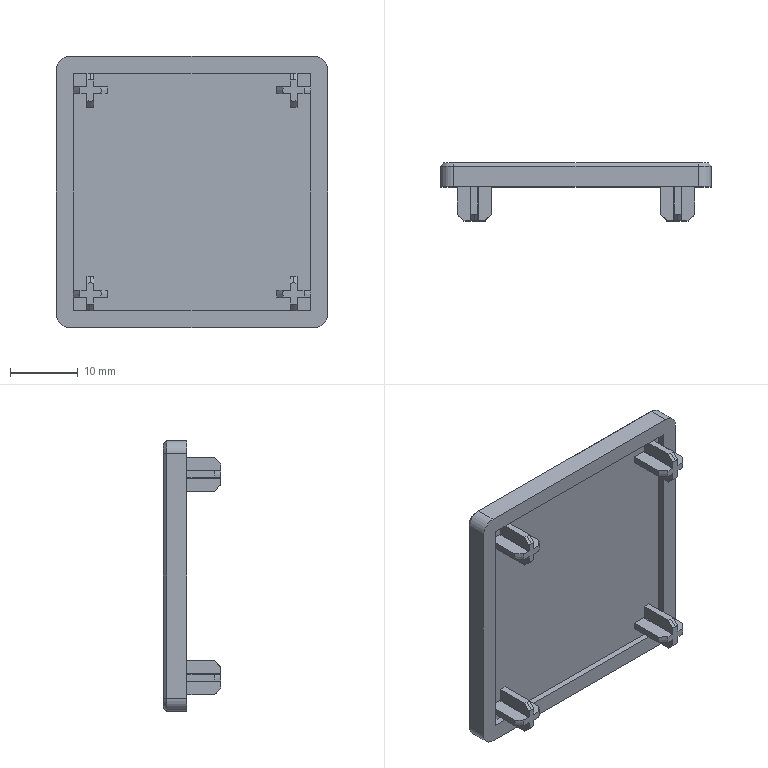Part | 1 solid | 123 faces | box 40 x 8.5 x 40 mm | volume 4553 mm3 | plane 79 | cone 24 | cylinder 20 | commonest cylinder face diameters 1.5 x16 4 x4